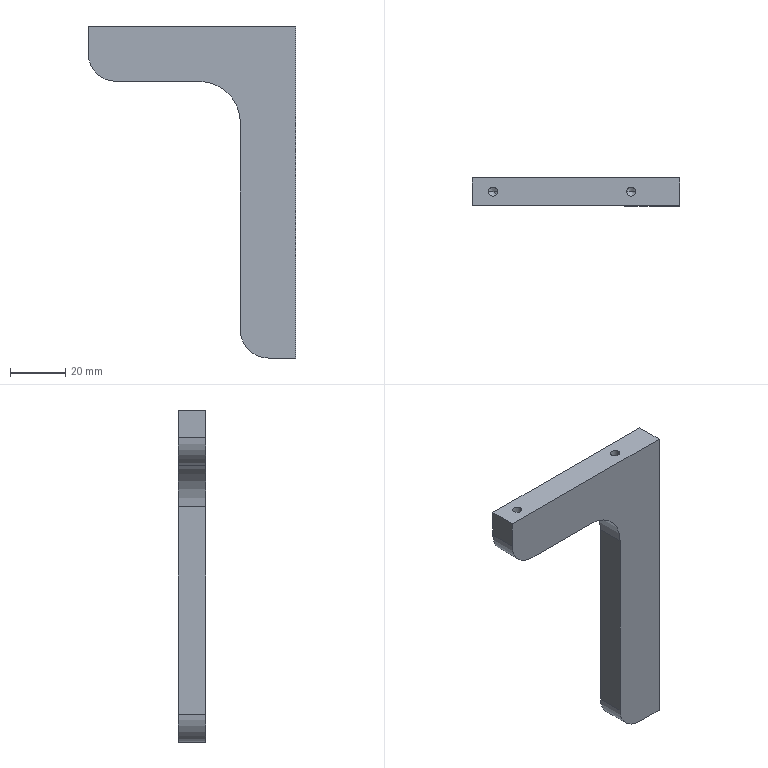Part | SolidWorks | features Fillet 2, HoleWzd 2, Extrusion 1, ICE 1 | 1 solid | 27 faces | box 75 x 10 x 120 mm | volume 34697 mm3 | cylinder 11 | cone 8 | plane 8 | commonest cylinder face diameters 3.3 x8 20 x2 30 x1
STEP:
#1=CARTESIAN_POINT('',(27.4,0.,29.15));
#2=VERTEX_POINT('',#1);
#3=CARTESIAN_POINT('',(27.4,0.,25.85));
#4=VERTEX_POINT('',#3);
#5=CARTESIAN_POINT('',(27.4,0.,27.5));
#6=DIRECTION('',(1.,0.,0.));
#7=DIRECTION('',(0.,0.,-1.));
#8=AXIS2_PLACEMENT_3D('',#5,#6,#7);
#9=CIRCLE('',#8,1.65);
#10=EDGE_CURVE('',#2,#4,#9,.T.);
#11=ORIENTED_EDGE('',*,*,#10,.F.);
#12=CARTESIAN_POINT('',(37.5,0.,29.15));
#13=VERTEX_POINT('',#12);
#14=CARTESIAN_POINT('',(37.5,0.,29.15));
#15=DIRECTION('',(1.,0.,0.));
#16=VECTOR('',#15,1000.);
#17=LINE('',#14,#16);
#18=EDGE_CURVE('',#2,#13,#17,.T.);
#19=ORIENTED_EDGE('',*,*,#18,.T.);
#20=CARTESIAN_POINT('',(37.5,0.,25.85));
#21=VERTEX_POINT('',#20);
#22=CARTESIAN_POINT('',(37.5,0.,27.5));
#23=DIRECTION('',(1.,0.,0.));
#24=DIRECTION('',(0.,0.,-1.));
#25=AXIS2_PLACEMENT_3D('',#22,#23,#24);
#26=CIRCLE('',#25,1.65);
#27=EDGE_CURVE('',#13,#21,#26,.T.);
#28=ORIENTED_EDGE('',*,*,#27,.T.);
#29=CARTESIAN_POINT('',(37.5,0.,25.85));
#30=DIRECTION('',(1.,0.,0.));
#31=VECTOR('',#30,1000.);
#32=LINE('',#29,#31);
#33=EDGE_CURVE('',#4,#21,#32,.T.);
#34=ORIENTED_EDGE('',*,*,#33,.F.);
#35=EDGE_LOOP('',(#11,#19,#28,#34));
#36=FACE_OUTER_BOUND('',#35,.T.);
#37=CARTESIAN_POINT('',(37.5,0.,27.5));
#38=DIRECTION('',(1.,0.,0.));
#39=DIRECTION('',(0.,0.,-1.));
#40=AXIS2_PLACEMENT_3D('',#37,#38,#39);
#41=CYLINDRICAL_SURFACE('',#40,1.65);
#42=ADVANCED_FACE('',(#36),#41,.F.);
#43=CARTESIAN_POINT('',(26.409,0.,27.5));
#44=VERTEX_POINT('',#43);
#45=CARTESIAN_POINT('',(27.4,0.,25.85));
#46=DIRECTION('',(0.515,0.,-0.8572));
#47=VECTOR('',#46,1000.);
#48=LINE('',#45,#47);
#49=EDGE_CURVE('',#44,#4,#48,.T.);
#50=ORIENTED_EDGE('',*,*,#49,.F.);
#51=CARTESIAN_POINT('',(27.4,0.,29.15));
#52=DIRECTION('',(0.515,0.,0.8572));
#53=VECTOR('',#52,1000.);
#54=LINE('',#51,#53);
#55=EDGE_CURVE('',#44,#2,#54,.T.);
#56=ORIENTED_EDGE('',*,*,#55,.T.);
#57=ORIENTED_EDGE('',*,*,#10,.T.);
#58=EDGE_LOOP('',(#50,#56,#57));
#59=FACE_OUTER_BOUND('',#58,.T.);
#60=CARTESIAN_POINT('',(27.4,0.,27.5));
#61=DIRECTION('',(1.,0.,0.));
#62=DIRECTION('',(0.,0.,-1.));
#63=AXIS2_PLACEMENT_3D('',#60,#61,#62);
#64=CONICAL_SURFACE('',#63,1.65,1.03);
#65=ADVANCED_FACE('',(#59),#64,.F.);
#66=CARTESIAN_POINT('',(27.4,0.,-50.85));
#67=VERTEX_POINT('',#66);
#68=CARTESIAN_POINT('',(27.4,0.,-54.15));
#69=VERTEX_POINT('',#68);
#70=CARTESIAN_POINT('',(27.4,0.,-52.5));
#71=DIRECTION('',(1.,0.,0.));
#72=DIRECTION('',(0.,0.,-1.));
#73=AXIS2_PLACEMENT_3D('',#70,#71,#72);
#74=CIRCLE('',#73,1.65);
#75=EDGE_CURVE('',#67,#69,#74,.T.);
#76=ORIENTED_EDGE('',*,*,#75,.F.);
#77=CARTESIAN_POINT('',(37.5,0.,-50.85));
#78=VERTEX_POINT('',#77);
#79=CARTESIAN_POINT('',(37.5,0.,-50.85));
#80=DIRECTION('',(1.,0.,0.));
#81=VECTOR('',#80,1000.);
#82=LINE('',#79,#81);
#83=EDGE_CURVE('',#67,#78,#82,.T.);
#84=ORIENTED_EDGE('',*,*,#83,.T.);
#85=CARTESIAN_POINT('',(37.5,0.,-54.15));
#86=VERTEX_POINT('',#85);
#87=CARTESIAN_POINT('',(37.5,0.,-52.5));
#88=DIRECTION('',(1.,0.,0.));
#89=DIRECTION('',(0.,0.,-1.));
#90=AXIS2_PLACEMENT_3D('',#87,#88,#89);
#91=CIRCLE('',#90,1.65);
#92=EDGE_CURVE('',#78,#86,#91,.T.);
#93=ORIENTED_EDGE('',*,*,#92,.T.);
#94=CARTESIAN_POINT('',(37.5,0.,-54.15));
#95=DIRECTION('',(1.,0.,0.));
#96=VECTOR('',#95,1000.);
#97=LINE('',#94,#96);
#98=EDGE_CURVE('',#69,#86,#97,.T.);
#99=ORIENTED_EDGE('',*,*,#98,.F.);
#100=EDGE_LOOP('',(#76,#84,#93,#99));
#101=FACE_OUTER_BOUND('',#100,.T.);
#102=CARTESIAN_POINT('',(37.5,0.,-52.5));
#103=DIRECTION('',(1.,0.,0.));
#104=DIRECTION('',(0.,0.,-1.));
#105=AXIS2_PLACEMENT_3D('',#102,#103,#104);
#106=CYLINDRICAL_SURFACE('',#105,1.65);
#107=ADVANCED_FACE('',(#101),#106,.F.);
#108=CARTESIAN_POINT('',(26.409,0.,-52.5));
#109=VERTEX_POINT('',#108);
#110=CARTESIAN_POINT('',(27.4,0.,-54.15));
#111=DIRECTION('',(0.515,0.,-0.8572));
#112=VECTOR('',#111,1000.);
#113=LINE('',#110,#112);
#114=EDGE_CURVE('',#109,#69,#113,.T.);
#115=ORIENTED_EDGE('',*,*,#114,.F.);
#116=CARTESIAN_POINT('',(27.4,0.,-50.85));
#117=DIRECTION('',(0.515,0.,0.8572));
#118=VECTOR('',#117,1000.);
#119=LINE('',#116,#118);
#120=EDGE_CURVE('',#109,#67,#119,.T.);
#121=ORIENTED_EDGE('',*,*,#120,.T.);
#122=ORIENTED_EDGE('',*,*,#75,.T.);
#123=EDGE_LOOP('',(#115,#121,#122));
#124=FACE_OUTER_BOUND('',#123,.T.);
#125=CARTESIAN_POINT('',(27.4,0.,-52.5));
#126=DIRECTION('',(1.,0.,0.));
#127=DIRECTION('',(0.,0.,-1.));
#128=AXIS2_PLACEMENT_3D('',#125,#126,#127);
#129=CONICAL_SURFACE('',#128,1.65,1.03);
#130=ADVANCED_FACE('',(#124),#129,.F.);
#131=CARTESIAN_POINT('',(-31.65,0.,49.9));
#132=VERTEX_POINT('',#131);
#133=CARTESIAN_POINT('',(-28.35,0.,49.9));
#134=VERTEX_POINT('',#133);
#135=CARTESIAN_POINT('',(-30.,0.,49.9));
#136=DIRECTION('',(0.,0.,1.));
#137=DIRECTION('',(1.,0.,0.));
#138=AXIS2_PLACEMENT_3D('',#135,#136,#137);
#139=CIRCLE('',#138,1.65);
#140=EDGE_CURVE('',#132,#134,#139,.T.);
#141=ORIENTED_EDGE('',*,*,#140,.F.);
#142=CARTESIAN_POINT('',(-31.65,0.,60.));
#143=VERTEX_POINT('',#142);
#144=CARTESIAN_POINT('',(-31.65,0.,60.));
#145=DIRECTION('',(0.,0.,1.));
#146=VECTOR('',#145,1000.);
#147=LINE('',#144,#146);
#148=EDGE_CURVE('',#132,#143,#147,.T.);
#149=ORIENTED_EDGE('',*,*,#148,.T.);
#150=CARTESIAN_POINT('',(-28.35,0.,60.));
#151=VERTEX_POINT('',#150);
#152=CARTESIAN_POINT('',(-30.,0.,60.));
#153=DIRECTION('',(0.,0.,1.));
#154=DIRECTION('',(1.,0.,0.));
#155=AXIS2_PLACEMENT_3D('',#152,#153,#154);
#156=CIRCLE('',#155,1.65);
#157=EDGE_CURVE('',#143,#151,#156,.T.);
#158=ORIENTED_EDGE('',*,*,#157,.T.);
#159=CARTESIAN_POINT('',(-28.35,0.,60.));
#160=DIRECTION('',(0.,0.,1.));
#161=VECTOR('',#160,1000.);
#162=LINE('',#159,#161);
#163=EDGE_CURVE('',#134,#151,#162,.T.);
#164=ORIENTED_EDGE('',*,*,#163,.F.);
#165=EDGE_LOOP('',(#141,#149,#158,#164));
#166=FACE_OUTER_BOUND('',#165,.T.);
#167=CARTESIAN_POINT('',(-30.,0.,60.));
#168=DIRECTION('',(0.,0.,1.));
#169=DIRECTION('',(1.,0.,0.));
#170=AXIS2_PLACEMENT_3D('',#167,#168,#169);
#171=CYLINDRICAL_SURFACE('',#170,1.65);
#172=ADVANCED_FACE('',(#166),#171,.F.);
#173=CARTESIAN_POINT('',(-30.,0.,48.909));
#174=VERTEX_POINT('',#173);
#175=CARTESIAN_POINT('',(-28.35,0.,49.9));
#176=DIRECTION('',(0.8572,0.,0.515));
#177=VECTOR('',#176,1000.);
#178=LINE('',#175,#177);
#179=EDGE_CURVE('',#174,#134,#178,.T.);
#180=ORIENTED_EDGE('',*,*,#179,.F.);
#181=CARTESIAN_POINT('',(-31.65,0.,49.9));
#182=DIRECTION('',(-0.8572,0.,0.515));
#183=VECTOR('',#182,1000.);
#184=LINE('',#181,#183);
#185=EDGE_CURVE('',#174,#132,#184,.T.);
#186=ORIENTED_EDGE('',*,*,#185,.T.);
#187=ORIENTED_EDGE('',*,*,#140,.T.);
#188=EDGE_LOOP('',(#180,#186,#187));
#189=FACE_OUTER_BOUND('',#188,.T.);
#190=CARTESIAN_POINT('',(-30.,0.,49.9));
#191=DIRECTION('',(0.,0.,1.));
#192=DIRECTION('',(1.,0.,0.));
#193=AXIS2_PLACEMENT_3D('',#190,#191,#192);
#194=CONICAL_SURFACE('',#193,1.65,1.03);
#195=ADVANCED_FACE('',(#189),#194,.F.);
#196=CARTESIAN_POINT('',(18.35,0.,49.9));
#197=VERTEX_POINT('',#196);
#198=CARTESIAN_POINT('',(21.65,0.,49.9));
#199=VERTEX_POINT('',#198);
#200=CARTESIAN_POINT('',(20.,0.,49.9));
#201=DIRECTION('',(0.,0.,1.));
#202=DIRECTION('',(1.,0.,0.));
#203=AXIS2_PLACEMENT_3D('',#200,#201,#202);
#204=CIRCLE('',#203,1.65);
#205=EDGE_CURVE('',#197,#199,#204,.T.);
#206=ORIENTED_EDGE('',*,*,#205,.F.);
#207=CARTESIAN_POINT('',(18.35,0.,60.));
#208=VERTEX_POINT('',#207);
#209=CARTESIAN_POINT('',(18.35,0.,60.));
#210=DIRECTION('',(0.,0.,1.));
#211=VECTOR('',#210,1000.);
#212=LINE('',#209,#211);
#213=EDGE_CURVE('',#197,#208,#212,.T.);
#214=ORIENTED_EDGE('',*,*,#213,.T.);
#215=CARTESIAN_POINT('',(21.65,0.,60.));
#216=VERTEX_POINT('',#215);
#217=CARTESIAN_POINT('',(20.,0.,60.));
#218=DIRECTION('',(0.,0.,1.));
#219=DIRECTION('',(1.,0.,0.));
#220=AXIS2_PLACEMENT_3D('',#217,#218,#219);
#221=CIRCLE('',#220,1.65);
#222=EDGE_CURVE('',#208,#216,#221,.T.);
#223=ORIENTED_EDGE('',*,*,#222,.T.);
#224=CARTESIAN_POINT('',(21.65,0.,60.));
#225=DIRECTION('',(0.,0.,1.));
#226=VECTOR('',#225,1000.);
#227=LINE('',#224,#226);
#228=EDGE_CURVE('',#199,#216,#227,.T.);
#229=ORIENTED_EDGE('',*,*,#228,.F.);
#230=EDGE_LOOP('',(#206,#214,#223,#229));
#231=FACE_OUTER_BOUND('',#230,.T.);
#232=CARTESIAN_POINT('',(20.,0.,60.));
#233=DIRECTION('',(0.,0.,1.));
#234=DIRECTION('',(1.,0.,0.));
#235=AXIS2_PLACEMENT_3D('',#232,#233,#234);
#236=CYLINDRICAL_SURFACE('',#235,1.65);
#237=ADVANCED_FACE('',(#231),#236,.F.);
#238=CARTESIAN_POINT('',(20.,0.,48.909));
#239=VERTEX_POINT('',#238);
#240=CARTESIAN_POINT('',(21.65,0.,49.9));
#241=DIRECTION('',(0.8572,0.,0.515));
#242=VECTOR('',#241,1000.);
#243=LINE('',#240,#242);
#244=EDGE_CURVE('',#239,#199,#243,.T.);
#245=ORIENTED_EDGE('',*,*,#244,.F.);
#246=CARTESIAN_POINT('',(18.35,0.,49.9));
#247=DIRECTION('',(-0.8572,0.,0.515));
#248=VECTOR('',#247,1000.);
#249=LINE('',#246,#248);
#250=EDGE_CURVE('',#239,#197,#249,.T.);
#251=ORIENTED_EDGE('',*,*,#250,.T.);
#252=ORIENTED_EDGE('',*,*,#205,.T.);
#253=EDGE_LOOP('',(#245,#251,#252));
#254=FACE_OUTER_BOUND('',#253,.T.);
#255=CARTESIAN_POINT('',(20.,0.,49.9));
#256=DIRECTION('',(0.,0.,1.));
#257=DIRECTION('',(1.,0.,0.));
#258=AXIS2_PLACEMENT_3D('',#255,#256,#257);
#259=CONICAL_SURFACE('',#258,1.65,1.03);
#260=ADVANCED_FACE('',(#254),#259,.F.);
#261=CARTESIAN_POINT('',(37.5,0.,27.5));
#262=DIRECTION('',(1.,0.,0.));
#263=DIRECTION('',(0.,0.,-1.));
#264=AXIS2_PLACEMENT_3D('',#261,#262,#263);
#265=CIRCLE('',#264,1.65);
#266=EDGE_CURVE('',#21,#13,#265,.T.);
#267=ORIENTED_EDGE('',*,*,#266,.F.);
#268=ORIENTED_EDGE('',*,*,#27,.F.);
#269=EDGE_LOOP('',(#267,#268));
#270=FACE_BOUND('',#269,.T.);
#271=CARTESIAN_POINT('',(37.5,0.,-52.5));
#272=DIRECTION('',(1.,0.,0.));
#273=DIRECTION('',(0.,0.,-1.));
#274=AXIS2_PLACEMENT_3D('',#271,#272,#273);
#275=CIRCLE('',#274,1.65);
#276=EDGE_CURVE('',#86,#78,#275,.T.);
#277=ORIENTED_EDGE('',*,*,#276,.F.);
#278=ORIENTED_EDGE('',*,*,#92,.F.);
#279=EDGE_LOOP('',(#277,#278));
#280=FACE_BOUND('',#279,.T.);
#281=CARTESIAN_POINT('',(37.5,-5.,60.));
#282=VERTEX_POINT('',#281);
#283=CARTESIAN_POINT('',(37.5,-5.,-60.));
#284=VERTEX_POINT('',#283);
#285=CARTESIAN_POINT('',(37.5,-5.,60.));
#286=DIRECTION('',(0.,0.,-1.));
#287=VECTOR('',#286,1000.);
#288=LINE('',#285,#287);
#289=EDGE_CURVE('',#282,#284,#288,.T.);
#290=ORIENTED_EDGE('',*,*,#289,.T.);
#291=CARTESIAN_POINT('',(37.5,5.,-60.));
#292=VERTEX_POINT('',#291);
#293=CARTESIAN_POINT('',(37.5,5.,-60.));
#294=DIRECTION('',(0.,-1.,0.));
#295=VECTOR('',#294,1000.);
#296=LINE('',#293,#295);
#297=EDGE_CURVE('',#292,#284,#296,.T.);
#298=ORIENTED_EDGE('',*,*,#297,.F.);
#299=CARTESIAN_POINT('',(37.5,5.,60.));
#300=VERTEX_POINT('',#299);
#301=CARTESIAN_POINT('',(37.5,5.,60.));
#302=DIRECTION('',(0.,0.,-1.));
#303=VECTOR('',#302,1000.);
#304=LINE('',#301,#303);
#305=EDGE_CURVE('',#300,#292,#304,.T.);
#306=ORIENTED_EDGE('',*,*,#305,.F.);
#307=CARTESIAN_POINT('',(37.5,5.,60.));
#308=DIRECTION('',(0.,-1.,0.));
#309=VECTOR('',#308,1000.);
#310=LINE('',#307,#309);
#311=EDGE_CURVE('',#300,#282,#310,.T.);
#312=ORIENTED_EDGE('',*,*,#311,.T.);
#313=EDGE_LOOP('',(#290,#298,#306,#312));
#314=FACE_OUTER_BOUND('',#313,.T.);
#315=CARTESIAN_POINT('',(37.5,5.,60.));
#316=DIRECTION('',(-1.,0.,0.));
#317=DIRECTION('',(0.,0.,1.));
#318=AXIS2_PLACEMENT_3D('',#315,#316,#317);
#319=PLANE('',#318);
#320=ADVANCED_FACE('',(#270,#280,#314),#319,.F.);
#321=CARTESIAN_POINT('',(27.5,-5.,-60.));
#322=VERTEX_POINT('',#321);
#323=CARTESIAN_POINT('',(-37.5,-5.,-60.));
#324=DIRECTION('',(-1.,0.,0.));
#325=VECTOR('',#324,1000.);
#326=LINE('',#323,#325);
#327=EDGE_CURVE('',#284,#322,#326,.T.);
#328=ORIENTED_EDGE('',*,*,#327,.T.);
#329=CARTESIAN_POINT('',(27.5,5.,-60.));
#330=VERTEX_POINT('',#329);
#331=CARTESIAN_POINT('',(27.5,5.,-60.));
#332=DIRECTION('',(0.,1.,0.));
#333=VECTOR('',#332,1000.);
#334=LINE('',#331,#333);
#335=EDGE_CURVE('',#322,#330,#334,.T.);
#336=ORIENTED_EDGE('',*,*,#335,.T.);
#337=CARTESIAN_POINT('',(-37.5,5.,-60.));
#338=DIRECTION('',(-1.,0.,0.));
#339=VECTOR('',#338,1000.);
#340=LINE('',#337,#339);
#341=EDGE_CURVE('',#292,#330,#340,.T.);
#342=ORIENTED_EDGE('',*,*,#341,.F.);
#343=ORIENTED_EDGE('',*,*,#297,.T.);
#344=EDGE_LOOP('',(#328,#336,#342,#343));
#345=FACE_OUTER_BOUND('',#344,.T.);
#346=CARTESIAN_POINT('',(-37.5,5.,-60.));
#347=DIRECTION('',(0.,0.,1.));
#348=DIRECTION('',(1.,0.,0.));
#349=AXIS2_PLACEMENT_3D('',#346,#347,#348);
#350=PLANE('',#349);
#351=ADVANCED_FACE('',(#345),#350,.F.);
#352=CARTESIAN_POINT('',(-37.5,5.,50.));
#353=VERTEX_POINT('',#352);
#354=CARTESIAN_POINT('',(-37.5,5.,60.));
#355=VERTEX_POINT('',#354);
#356=CARTESIAN_POINT('',(-37.5,5.,60.));
#357=DIRECTION('',(0.,0.,1.));
#358=VECTOR('',#357,1000.);
#359=LINE('',#356,#358);
#360=EDGE_CURVE('',#353,#355,#359,.T.);
#361=ORIENTED_EDGE('',*,*,#360,.F.);
#362=CARTESIAN_POINT('',(-37.5,-5.,50.));
#363=VERTEX_POINT('',#362);
#364=CARTESIAN_POINT('',(-37.5,5.,50.));
#365=DIRECTION('',(0.,-1.,0.));
#366=VECTOR('',#365,1000.);
#367=LINE('',#364,#366);
#368=EDGE_CURVE('',#353,#363,#367,.T.);
#369=ORIENTED_EDGE('',*,*,#368,.T.);
#370=CARTESIAN_POINT('',(-37.5,-5.,60.));
#371=VERTEX_POINT('',#370);
#372=CARTESIAN_POINT('',(-37.5,-5.,60.));
#373=DIRECTION('',(0.,0.,1.));
#374=VECTOR('',#373,1000.);
#375=LINE('',#372,#374);
#376=EDGE_CURVE('',#363,#371,#375,.T.);
#377=ORIENTED_EDGE('',*,*,#376,.T.);
#378=CARTESIAN_POINT('',(-37.5,5.,60.));
#379=DIRECTION('',(0.,-1.,0.));
#380=VECTOR('',#379,1000.);
#381=LINE('',#378,#380);
#382=EDGE_CURVE('',#355,#371,#381,.T.);
#383=ORIENTED_EDGE('',*,*,#382,.F.);
#384=EDGE_LOOP('',(#361,#369,#377,#383));
#385=FACE_OUTER_BOUND('',#384,.T.);
#386=CARTESIAN_POINT('',(-37.5,5.,60.));
#387=DIRECTION('',(1.,0.,0.));
#388=DIRECTION('',(0.,0.,-1.));
#389=AXIS2_PLACEMENT_3D('',#386,#387,#388);
#390=PLANE('',#389);
#391=ADVANCED_FACE('',(#385),#390,.F.);
#392=CARTESIAN_POINT('',(-30.,0.,60.));
#393=DIRECTION('',(0.,0.,1.));
#394=DIRECTION('',(1.,0.,0.));
#395=AXIS2_PLACEMENT_3D('',#392,#393,#394);
#396=CIRCLE('',#395,1.65);
#397=EDGE_CURVE('',#151,#143,#396,.T.);
#398=ORIENTED_EDGE('',*,*,#397,.F.);
#399=ORIENTED_EDGE('',*,*,#157,.F.);
#400=EDGE_LOOP('',(#398,#399));
#401=FACE_BOUND('',#400,.T.);
#402=CARTESIAN_POINT('',(20.,0.,60.));
#403=DIRECTION('',(0.,0.,1.));
#404=DIRECTION('',(1.,0.,0.));
#405=AXIS2_PLACEMENT_3D('',#402,#403,#404);
#406=CIRCLE('',#405,1.65);
#407=EDGE_CURVE('',#216,#208,#406,.T.);
#408=ORIENTED_EDGE('',*,*,#407,.F.);
#409=ORIENTED_EDGE('',*,*,#222,.F.);
#410=EDGE_LOOP('',(#408,#409));
#411=FACE_BOUND('',#410,.T.);
#412=CARTESIAN_POINT('',(-37.5,-5.,60.));
#413=DIRECTION('',(1.,0.,0.));
#414=VECTOR('',#413,1000.);
#415=LINE('',#412,#414);
#416=EDGE_CURVE('',#371,#282,#415,.T.);
#417=ORIENTED_EDGE('',*,*,#416,.T.);
#418=ORIENTED_EDGE('',*,*,#311,.F.);
#419=CARTESIAN_POINT('',(-37.5,5.,60.));
#420=DIRECTION('',(1.,0.,0.));
#421=VECTOR('',#420,1000.);
#422=LINE('',#419,#421);
#423=EDGE_CURVE('',#355,#300,#422,.T.);
#424=ORIENTED_EDGE('',*,*,#423,.F.);
#425=ORIENTED_EDGE('',*,*,#382,.T.);
#426=EDGE_LOOP('',(#417,#418,#424,#425));
#427=FACE_OUTER_BOUND('',#426,.T.);
#428=CARTESIAN_POINT('',(-37.5,5.,60.));
#429=DIRECTION('',(0.,0.,-1.));
#430=DIRECTION('',(-1.,0.,0.));
#431=AXIS2_PLACEMENT_3D('',#428,#429,#430);
#432=PLANE('',#431);
#433=ADVANCED_FACE('',(#401,#411,#427),#432,.F.);
#434=ORIENTED_EDGE('',*,*,#341,.T.);
#435=CARTESIAN_POINT('',(17.5,5.,-50.));
#436=VERTEX_POINT('',#435);
#437=CARTESIAN_POINT('',(27.5,5.,-50.));
#438=DIRECTION('',(0.,1.,0.));
#439=DIRECTION('',(0.,0.,-1.));
#440=AXIS2_PLACEMENT_3D('',#437,#438,#439);
#441=CIRCLE('',#440,10.);
#442=EDGE_CURVE('',#330,#436,#441,.T.);
#443=ORIENTED_EDGE('',*,*,#442,.T.);
#444=CARTESIAN_POINT('',(17.5,5.,25.));
#445=VERTEX_POINT('',#444);
#446=CARTESIAN_POINT('',(17.5,5.,-60.));
#447=DIRECTION('',(0.,0.,-1.));
#448=VECTOR('',#447,1000.);
#449=LINE('',#446,#448);
#450=EDGE_CURVE('',#445,#436,#449,.T.);
#451=ORIENTED_EDGE('',*,*,#450,.F.);
#452=CARTESIAN_POINT('',(2.5,5.,40.));
#453=VERTEX_POINT('',#452);
#454=CARTESIAN_POINT('',(2.5,5.,25.));
#455=DIRECTION('',(0.,-1.,0.));
#456=DIRECTION('',(0.,0.,-1.));
#457=AXIS2_PLACEMENT_3D('',#454,#455,#456);
#458=CIRCLE('',#457,15.);
#459=EDGE_CURVE('',#445,#453,#458,.T.);
#460=ORIENTED_EDGE('',*,*,#459,.T.);
#461=CARTESIAN_POINT('',(-27.5,5.,40.));
#462=VERTEX_POINT('',#461);
#463=CARTESIAN_POINT('',(-37.5,5.,40.));
#464=DIRECTION('',(1.,0.,0.));
#465=VECTOR('',#464,1000.);
#466=LINE('',#463,#465);
#467=EDGE_CURVE('',#462,#453,#466,.T.);
#468=ORIENTED_EDGE('',*,*,#467,.F.);
#469=CARTESIAN_POINT('',(-27.5,5.,50.));
#470=DIRECTION('',(0.,1.,0.));
#471=DIRECTION('',(0.,0.,-1.));
#472=AXIS2_PLACEMENT_3D('',#469,#470,#471);
#473=CIRCLE('',#472,10.);
#474=EDGE_CURVE('',#462,#353,#473,.T.);
#475=ORIENTED_EDGE('',*,*,#474,.T.);
#476=ORIENTED_EDGE('',*,*,#360,.T.);
#477=ORIENTED_EDGE('',*,*,#423,.T.);
#478=ORIENTED_EDGE('',*,*,#305,.T.);
#479=EDGE_LOOP('',(#434,#443,#451,#460,#468,#475,#476,#477,#478));
#480=FACE_OUTER_BOUND('',#479,.T.);
#481=CARTESIAN_POINT('',(0.,5.,0.));
#482=DIRECTION('',(0.,-1.,0.));
#483=DIRECTION('',(0.,0.,-1.));
#484=AXIS2_PLACEMENT_3D('',#481,#482,#483);
#485=PLANE('',#484);
#486=ADVANCED_FACE('',(#480),#485,.F.);
#487=CARTESIAN_POINT('',(17.5,-5.,25.));
#488=VERTEX_POINT('',#487);
#489=CARTESIAN_POINT('',(17.5,-5.,-50.));
#490=VERTEX_POINT('',#489);
#491=CARTESIAN_POINT('',(17.5,-5.,-60.));
#492=DIRECTION('',(0.,0.,-1.));
#493=VECTOR('',#492,1000.);
#494=LINE('',#491,#493);
#495=EDGE_CURVE('',#488,#490,#494,.T.);
#496=ORIENTED_EDGE('',*,*,#495,.T.);
#497=CARTESIAN_POINT('',(27.5,-5.,-50.));
#498=DIRECTION('',(0.,-1.,0.));
#499=DIRECTION('',(0.,0.,-1.));
#500=AXIS2_PLACEMENT_3D('',#497,#498,#499);
#501=CIRCLE('',#500,10.);
#502=EDGE_CURVE('',#490,#322,#501,.T.);
#503=ORIENTED_EDGE('',*,*,#502,.T.);
#504=ORIENTED_EDGE('',*,*,#327,.F.);
#505=ORIENTED_EDGE('',*,*,#289,.F.);
#506=ORIENTED_EDGE('',*,*,#416,.F.);
#507=ORIENTED_EDGE('',*,*,#376,.F.);
#508=CARTESIAN_POINT('',(-27.5,-5.,40.));
#509=VERTEX_POINT('',#508);
#510=CARTESIAN_POINT('',(-27.5,-5.,50.));
#511=DIRECTION('',(0.,-1.,0.));
#512=DIRECTION('',(0.,0.,-1.));
#513=AXIS2_PLACEMENT_3D('',#510,#511,#512);
#514=CIRCLE('',#513,10.);
#515=EDGE_CURVE('',#363,#509,#514,.T.);
#516=ORIENTED_EDGE('',*,*,#515,.T.);
#517=CARTESIAN_POINT('',(2.5,-5.,40.));
#518=VERTEX_POINT('',#517);
#519=CARTESIAN_POINT('',(-37.5,-5.,40.));
#520=DIRECTION('',(1.,0.,0.));
#521=VECTOR('',#520,1000.);
#522=LINE('',#519,#521);
#523=EDGE_CURVE('',#509,#518,#522,.T.);
#524=ORIENTED_EDGE('',*,*,#523,.T.);
#525=CARTESIAN_POINT('',(2.5,-5.,25.));
#526=DIRECTION('',(0.,1.,0.));
#527=DIRECTION('',(0.,0.,-1.));
#528=AXIS2_PLACEMENT_3D('',#525,#526,#527);
#529=CIRCLE('',#528,15.);
#530=EDGE_CURVE('',#518,#488,#529,.T.);
#531=ORIENTED_EDGE('',*,*,#530,.T.);
#532=EDGE_LOOP('',(#496,#503,#504,#505,#506,#507,#516,#524,#531));
#533=FACE_OUTER_BOUND('',#532,.T.);
#534=CARTESIAN_POINT('',(0.,-5.,0.));
#535=DIRECTION('',(0.,-1.,0.));
#536=DIRECTION('',(0.,0.,-1.));
#537=AXIS2_PLACEMENT_3D('',#534,#535,#536);
#538=PLANE('',#537);
#539=ADVANCED_FACE('',(#533),#538,.T.);
#540=ORIENTED_EDGE('',*,*,#523,.F.);
#541=CARTESIAN_POINT('',(-27.5,-119.127,40.));
#542=DIRECTION('',(0.,1.,0.));
#543=VECTOR('',#542,1000.);
#544=LINE('',#541,#543);
#545=EDGE_CURVE('',#509,#462,#544,.T.);
#546=ORIENTED_EDGE('',*,*,#545,.T.);
#547=ORIENTED_EDGE('',*,*,#467,.T.);
#548=CARTESIAN_POINT('',(2.5,-5.,40.));
#549=DIRECTION('',(0.,-1.,0.));
#550=VECTOR('',#549,1000.);
#551=LINE('',#548,#550);
#552=EDGE_CURVE('',#453,#518,#551,.T.);
#553=ORIENTED_EDGE('',*,*,#552,.T.);
#554=EDGE_LOOP('',(#540,#546,#547,#553));
#555=FACE_OUTER_BOUND('',#554,.T.);
#556=CARTESIAN_POINT('',(-37.5,-119.127,40.));
#557=DIRECTION('',(0.,0.,1.));
#558=DIRECTION('',(1.,0.,0.));
#559=AXIS2_PLACEMENT_3D('',#556,#557,#558);
#560=PLANE('',#559);
#561=ADVANCED_FACE('',(#555),#560,.F.);
#562=ORIENTED_EDGE('',*,*,#450,.T.);
#563=CARTESIAN_POINT('',(17.5,-119.127,-50.));
#564=DIRECTION('',(0.,-1.,0.));
#565=VECTOR('',#564,1000.);
#566=LINE('',#563,#565);
#567=EDGE_CURVE('',#436,#490,#566,.T.);
#568=ORIENTED_EDGE('',*,*,#567,.T.);
#569=ORIENTED_EDGE('',*,*,#495,.F.);
#570=CARTESIAN_POINT('',(17.5,5.,25.));
#571=DIRECTION('',(0.,1.,0.));
#572=VECTOR('',#571,1000.);
#573=LINE('',#570,#572);
#574=EDGE_CURVE('',#488,#445,#573,.T.);
#575=ORIENTED_EDGE('',*,*,#574,.T.);
#576=EDGE_LOOP('',(#562,#568,#569,#575));
#577=FACE_OUTER_BOUND('',#576,.T.);
#578=CARTESIAN_POINT('',(17.5,-119.127,-60.));
#579=DIRECTION('',(1.,0.,0.));
#580=DIRECTION('',(0.,0.,-1.));
#581=AXIS2_PLACEMENT_3D('',#578,#579,#580);
#582=PLANE('',#581);
#583=ADVANCED_FACE('',(#577),#582,.F.);
#584=ORIENTED_EDGE('',*,*,#530,.F.);
#585=ORIENTED_EDGE('',*,*,#552,.F.);
#586=ORIENTED_EDGE('',*,*,#459,.F.);
#587=ORIENTED_EDGE('',*,*,#574,.F.);
#588=EDGE_LOOP('',(#584,#585,#586,#587));
#589=FACE_OUTER_BOUND('',#588,.T.);
#590=CARTESIAN_POINT('',(2.5,-119.127,25.));
#591=DIRECTION('',(0.,-1.,0.));
#592=DIRECTION('',(0.,0.,-1.));
#593=AXIS2_PLACEMENT_3D('',#590,#591,#592);
#594=CYLINDRICAL_SURFACE('',#593,15.);
#595=ADVANCED_FACE('',(#589),#594,.F.);
#596=ORIENTED_EDGE('',*,*,#502,.F.);
#597=ORIENTED_EDGE('',*,*,#567,.F.);
#598=ORIENTED_EDGE('',*,*,#442,.F.);
#599=ORIENTED_EDGE('',*,*,#335,.F.);
#600=EDGE_LOOP('',(#596,#597,#598,#599));
#601=FACE_OUTER_BOUND('',#600,.T.);
#602=CARTESIAN_POINT('',(27.5,5.,-50.));
#603=DIRECTION('',(0.,1.,0.));
#604=DIRECTION('',(0.,0.,1.));
#605=AXIS2_PLACEMENT_3D('',#602,#603,#604);
#606=CYLINDRICAL_SURFACE('',#605,10.);
#607=ADVANCED_FACE('',(#601),#606,.T.);
#608=ORIENTED_EDGE('',*,*,#515,.F.);
#609=ORIENTED_EDGE('',*,*,#368,.F.);
#610=ORIENTED_EDGE('',*,*,#474,.F.);
#611=ORIENTED_EDGE('',*,*,#545,.F.);
#612=EDGE_LOOP('',(#608,#609,#610,#611));
#613=FACE_OUTER_BOUND('',#612,.T.);
#614=CARTESIAN_POINT('',(-27.5,-119.127,50.));
#615=DIRECTION('',(0.,1.,0.));
#616=DIRECTION('',(0.,0.,1.));
#617=AXIS2_PLACEMENT_3D('',#614,#615,#616);
#618=CYLINDRICAL_SURFACE('',#617,10.);
#619=ADVANCED_FACE('',(#613),#618,.T.);
#620=ORIENTED_EDGE('',*,*,#250,.F.);
#621=ORIENTED_EDGE('',*,*,#244,.T.);
#622=CARTESIAN_POINT('',(20.,0.,49.9));
#623=DIRECTION('',(0.,0.,1.));
#624=DIRECTION('',(1.,0.,0.));
#625=AXIS2_PLACEMENT_3D('',#622,#623,#624);
#626=CIRCLE('',#625,1.65);
#627=EDGE_CURVE('',#199,#197,#626,.T.);
#628=ORIENTED_EDGE('',*,*,#627,.T.);
#629=EDGE_LOOP('',(#620,#621,#628));
#630=FACE_OUTER_BOUND('',#629,.T.);
#631=CARTESIAN_POINT('',(20.,0.,49.9));
#632=DIRECTION('',(0.,0.,1.));
#633=DIRECTION('',(1.,0.,0.));
#634=AXIS2_PLACEMENT_3D('',#631,#632,#633);
#635=CONICAL_SURFACE('',#634,1.65,1.03);
#636=ADVANCED_FACE('',(#630),#635,.F.);
#637=ORIENTED_EDGE('',*,*,#213,.F.);
#638=ORIENTED_EDGE('',*,*,#627,.F.);
#639=ORIENTED_EDGE('',*,*,#228,.T.);
#640=ORIENTED_EDGE('',*,*,#407,.T.);
#641=EDGE_LOOP('',(#637,#638,#639,#640));
#642=FACE_OUTER_BOUND('',#641,.T.);
#643=CARTESIAN_POINT('',(20.,0.,60.));
#644=DIRECTION('',(0.,0.,1.));
#645=DIRECTION('',(1.,0.,0.));
#646=AXIS2_PLACEMENT_3D('',#643,#644,#645);
#647=CYLINDRICAL_SURFACE('',#646,1.65);
#648=ADVANCED_FACE('',(#642),#647,.F.);
#649=ORIENTED_EDGE('',*,*,#185,.F.);
#650=ORIENTED_EDGE('',*,*,#179,.T.);
#651=CARTESIAN_POINT('',(-30.,0.,49.9));
#652=DIRECTION('',(0.,0.,1.));
#653=DIRECTION('',(1.,0.,0.));
#654=AXIS2_PLACEMENT_3D('',#651,#652,#653);
#655=CIRCLE('',#654,1.65);
#656=EDGE_CURVE('',#134,#132,#655,.T.);
#657=ORIENTED_EDGE('',*,*,#656,.T.);
#658=EDGE_LOOP('',(#649,#650,#657));
#659=FACE_OUTER_BOUND('',#658,.T.);
#660=CARTESIAN_POINT('',(-30.,0.,49.9));
#661=DIRECTION('',(0.,0.,1.));
#662=DIRECTION('',(1.,0.,0.));
#663=AXIS2_PLACEMENT_3D('',#660,#661,#662);
#664=CONICAL_SURFACE('',#663,1.65,1.03);
#665=ADVANCED_FACE('',(#659),#664,.F.);
#666=ORIENTED_EDGE('',*,*,#148,.F.);
#667=ORIENTED_EDGE('',*,*,#656,.F.);
#668=ORIENTED_EDGE('',*,*,#163,.T.);
#669=ORIENTED_EDGE('',*,*,#397,.T.);
#670=EDGE_LOOP('',(#666,#667,#668,#669));
#671=FACE_OUTER_BOUND('',#670,.T.);
#672=CARTESIAN_POINT('',(-30.,0.,60.));
#673=DIRECTION('',(0.,0.,1.));
#674=DIRECTION('',(1.,0.,0.));
#675=AXIS2_PLACEMENT_3D('',#672,#673,#674);
#676=CYLINDRICAL_SURFACE('',#675,1.65);
#677=ADVANCED_FACE('',(#671),#676,.F.);
#678=ORIENTED_EDGE('',*,*,#120,.F.);
#679=ORIENTED_EDGE('',*,*,#114,.T.);
#680=CARTESIAN_POINT('',(27.4,0.,-52.5));
#681=DIRECTION('',(1.,0.,0.));
#682=DIRECTION('',(0.,0.,-1.));
#683=AXIS2_PLACEMENT_3D('',#680,#681,#682);
#684=CIRCLE('',#683,1.65);
#685=EDGE_CURVE('',#69,#67,#684,.T.);
#686=ORIENTED_EDGE('',*,*,#685,.T.);
#687=EDGE_LOOP('',(#678,#679,#686));
#688=FACE_OUTER_BOUND('',#687,.T.);
#689=CARTESIAN_POINT('',(27.4,0.,-52.5));
#690=DIRECTION('',(1.,0.,0.));
#691=DIRECTION('',(0.,0.,-1.));
#692=AXIS2_PLACEMENT_3D('',#689,#690,#691);
#693=CONICAL_SURFACE('',#692,1.65,1.03);
#694=ADVANCED_FACE('',(#688),#693,.F.);
#695=ORIENTED_EDGE('',*,*,#83,.F.);
#696=ORIENTED_EDGE('',*,*,#685,.F.);
#697=ORIENTED_EDGE('',*,*,#98,.T.);
#698=ORIENTED_EDGE('',*,*,#276,.T.);
#699=EDGE_LOOP('',(#695,#696,#697,#698));
#700=FACE_OUTER_BOUND('',#699,.T.);
#701=CARTESIAN_POINT('',(37.5,0.,-52.5));
#702=DIRECTION('',(1.,0.,0.));
#703=DIRECTION('',(0.,0.,-1.));
#704=AXIS2_PLACEMENT_3D('',#701,#702,#703);
#705=CYLINDRICAL_SURFACE('',#704,1.65);
#706=ADVANCED_FACE('',(#700),#705,.F.);
#707=ORIENTED_EDGE('',*,*,#55,.F.);
#708=ORIENTED_EDGE('',*,*,#49,.T.);
#709=CARTESIAN_POINT('',(27.4,0.,27.5));
#710=DIRECTION('',(1.,0.,0.));
#711=DIRECTION('',(0.,0.,-1.));
#712=AXIS2_PLACEMENT_3D('',#709,#710,#711);
#713=CIRCLE('',#712,1.65);
#714=EDGE_CURVE('',#4,#2,#713,.T.);
#715=ORIENTED_EDGE('',*,*,#714,.T.);
#716=EDGE_LOOP('',(#707,#708,#715));
#717=FACE_OUTER_BOUND('',#716,.T.);
#718=CARTESIAN_POINT('',(27.4,0.,27.5));
#719=DIRECTION('',(1.,0.,0.));
#720=DIRECTION('',(0.,0.,-1.));
#721=AXIS2_PLACEMENT_3D('',#718,#719,#720);
#722=CONICAL_SURFACE('',#721,1.65,1.03);
#723=ADVANCED_FACE('',(#717),#722,.F.);
#724=ORIENTED_EDGE('',*,*,#18,.F.);
#725=ORIENTED_EDGE('',*,*,#714,.F.);
#726=ORIENTED_EDGE('',*,*,#33,.T.);
#727=ORIENTED_EDGE('',*,*,#266,.T.);
#728=EDGE_LOOP('',(#724,#725,#726,#727));
#729=FACE_OUTER_BOUND('',#728,.T.);
#730=CARTESIAN_POINT('',(37.5,0.,27.5));
#731=DIRECTION('',(1.,0.,0.));
#732=DIRECTION('',(0.,0.,-1.));
#733=AXIS2_PLACEMENT_3D('',#730,#731,#732);
#734=CYLINDRICAL_SURFACE('',#733,1.65);
#735=ADVANCED_FACE('',(#729),#734,.F.);
#736=CLOSED_SHELL('',(#42,#65,#107,#130,#172,#195,#237,#260,#320,#351,#391,#433,#486,#539,#561,#583,#595,#607,#619,#636,#648,#665,#677,#694,#706,#723,#735));
#737=MANIFOLD_SOLID_BREP('',#736);
#738=CARTESIAN_POINT('',(0.,0.,0.));
#739=DIRECTION('',(0.,0.,1.));
#740=DIRECTION('',(1.,0.,0.));
#741=AXIS2_PLACEMENT_3D('',#738,#739,#740);
#742=(LENGTH_UNIT()NAMED_UNIT(*)SI_UNIT(.MILLI.,.METRE.));
#743=UNCERTAINTY_MEASURE_WITH_UNIT(LENGTH_MEASURE(0.00001),#742,'','');
#744=(NAMED_UNIT(*)PLANE_ANGLE_UNIT()SI_UNIT($,.RADIAN.));
#745=(NAMED_UNIT(*)SI_UNIT($,.STERADIAN.)SOLID_ANGLE_UNIT());
#746=(GEOMETRIC_REPRESENTATION_CONTEXT(3)GLOBAL_UNCERTAINTY_ASSIGNED_CONTEXT((#743))GLOBAL_UNIT_ASSIGNED_CONTEXT((#742,#744,#745))REPRESENTATION_CONTEXT('',''));
#747=ADVANCED_BREP_SHAPE_REPRESENTATION('',(#737,#741),#746);